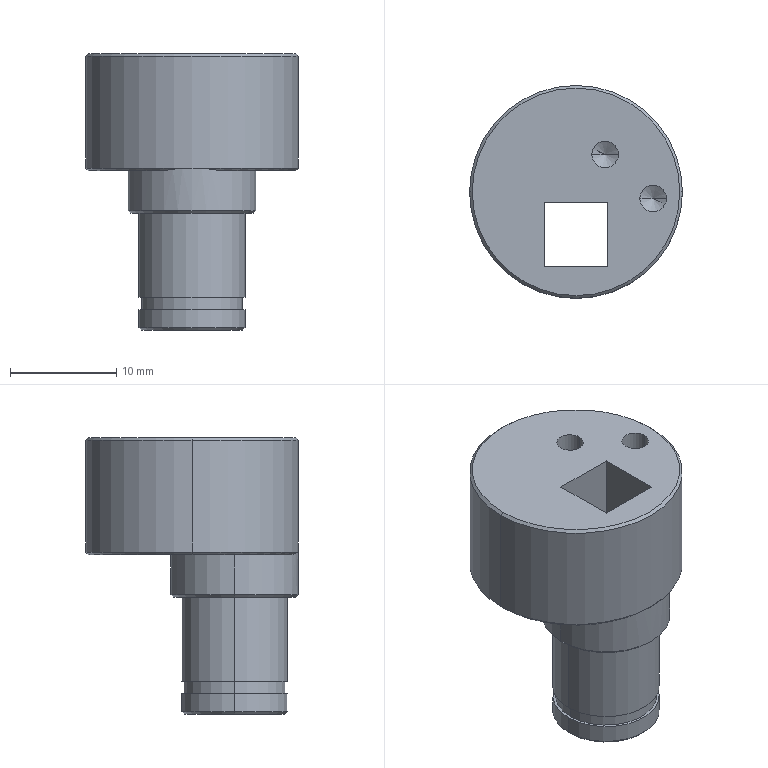Part | NX | features BREP 1 | 1 solid | 37 faces | box 20 x 20 x 26 mm | volume 3745 mm3 | cylinder 14 | cone 13 | plane 10 | commonest cylinder face diameters 2.5 x4 10 x4 9.5 x2 12 x2 20 x2
STEP:
#1=CARTESIAN_POINT('',(1.486,3.518,11.));
#2=VERTEX_POINT('',#1);
#3=CARTESIAN_POINT('',(1.486,3.518,3.5));
#4=VERTEX_POINT('',#3);
#5=CARTESIAN_POINT('',(1.486,3.518,11.));
#6=DIRECTION('',(0.,0.,1.));
#7=VECTOR('',#6,1000.);
#8=LINE('',#5,#7);
#9=EDGE_CURVE('',#2,#4,#8,.F.);
#10=ORIENTED_EDGE('',*,*,#9,.T.);
#11=CARTESIAN_POINT('',(3.986,3.518,3.5));
#12=VERTEX_POINT('',#11);
#13=CARTESIAN_POINT('',(2.736,3.518,3.5));
#14=DIRECTION('',(0.,0.,1.));
#15=DIRECTION('',(1.,0.,0.));
#16=AXIS2_PLACEMENT_3D('',#13,#14,#15);
#17=CIRCLE('',#16,1.25);
#18=EDGE_CURVE('',#12,#4,#17,.T.);
#19=ORIENTED_EDGE('',*,*,#18,.F.);
#20=CARTESIAN_POINT('',(3.986,3.518,11.));
#21=VERTEX_POINT('',#20);
#22=CARTESIAN_POINT('',(3.986,3.518,11.));
#23=DIRECTION('',(0.,0.,1.));
#24=VECTOR('',#23,1000.);
#25=LINE('',#22,#24);
#26=EDGE_CURVE('',#21,#12,#25,.F.);
#27=ORIENTED_EDGE('',*,*,#26,.F.);
#28=CARTESIAN_POINT('',(2.736,3.518,11.));
#29=DIRECTION('',(0.,0.,1.));
#30=DIRECTION('',(1.,0.,0.));
#31=AXIS2_PLACEMENT_3D('',#28,#29,#30);
#32=CIRCLE('',#31,1.25);
#33=EDGE_CURVE('',#21,#2,#32,.T.);
#34=ORIENTED_EDGE('',*,*,#33,.T.);
#35=EDGE_LOOP('',(#10,#19,#27,#34));
#36=FACE_BOUND('',#35,.T.);
#37=CARTESIAN_POINT('',(2.736,3.518,11.));
#38=DIRECTION('',(0.,0.,1.));
#39=DIRECTION('',(1.,0.,0.));
#40=AXIS2_PLACEMENT_3D('',#37,#38,#39);
#41=CYLINDRICAL_SURFACE('',#40,1.25);
#42=ADVANCED_FACE('',(#36),#41,.F.);
#43=CARTESIAN_POINT('',(2.736,3.518,2.749));
#44=VERTEX_POINT('',#43);
#45=CARTESIAN_POINT('',(1.486,3.518,3.5));
#46=DIRECTION('',(-0.8572,0.,0.515));
#47=VECTOR('',#46,1000.);
#48=LINE('',#45,#47);
#49=EDGE_CURVE('',#44,#4,#48,.T.);
#50=ORIENTED_EDGE('',*,*,#49,.F.);
#51=CARTESIAN_POINT('',(3.986,3.518,3.5));
#52=DIRECTION('',(0.8572,0.,0.515));
#53=VECTOR('',#52,1000.);
#54=LINE('',#51,#53);
#55=EDGE_CURVE('',#44,#12,#54,.T.);
#56=ORIENTED_EDGE('',*,*,#55,.T.);
#57=ORIENTED_EDGE('',*,*,#18,.T.);
#58=EDGE_LOOP('',(#50,#56,#57));
#59=FACE_BOUND('',#58,.T.);
#60=CARTESIAN_POINT('',(2.736,3.518,3.5));
#61=DIRECTION('',(0.,0.,1.));
#62=DIRECTION('',(1.,0.,0.));
#63=AXIS2_PLACEMENT_3D('',#60,#61,#62);
#64=CONICAL_SURFACE('',#63,1.25,1.03);
#65=ADVANCED_FACE('',(#59),#64,.F.);
#66=CARTESIAN_POINT('',(6.,-0.6191,11.));
#67=VERTEX_POINT('',#66);
#68=CARTESIAN_POINT('',(6.,-0.6191,3.5));
#69=VERTEX_POINT('',#68);
#70=CARTESIAN_POINT('',(6.,-0.6191,11.));
#71=DIRECTION('',(0.,0.,1.));
#72=VECTOR('',#71,1000.);
#73=LINE('',#70,#72);
#74=EDGE_CURVE('',#67,#69,#73,.F.);
#75=ORIENTED_EDGE('',*,*,#74,.T.);
#76=CARTESIAN_POINT('',(8.5,-0.6191,3.5));
#77=VERTEX_POINT('',#76);
#78=CARTESIAN_POINT('',(7.25,-0.6191,3.5));
#79=DIRECTION('',(0.,0.,1.));
#80=DIRECTION('',(1.,0.,0.));
#81=AXIS2_PLACEMENT_3D('',#78,#79,#80);
#82=CIRCLE('',#81,1.25);
#83=EDGE_CURVE('',#77,#69,#82,.T.);
#84=ORIENTED_EDGE('',*,*,#83,.F.);
#85=CARTESIAN_POINT('',(8.5,-0.6191,11.));
#86=VERTEX_POINT('',#85);
#87=CARTESIAN_POINT('',(8.5,-0.6191,11.));
#88=DIRECTION('',(0.,0.,1.));
#89=VECTOR('',#88,1000.);
#90=LINE('',#87,#89);
#91=EDGE_CURVE('',#86,#77,#90,.F.);
#92=ORIENTED_EDGE('',*,*,#91,.F.);
#93=CARTESIAN_POINT('',(7.25,-0.6191,11.));
#94=DIRECTION('',(0.,0.,1.));
#95=DIRECTION('',(1.,0.,0.));
#96=AXIS2_PLACEMENT_3D('',#93,#94,#95);
#97=CIRCLE('',#96,1.25);
#98=EDGE_CURVE('',#86,#67,#97,.T.);
#99=ORIENTED_EDGE('',*,*,#98,.T.);
#100=EDGE_LOOP('',(#75,#84,#92,#99));
#101=FACE_BOUND('',#100,.T.);
#102=CARTESIAN_POINT('',(7.25,-0.6191,11.));
#103=DIRECTION('',(0.,0.,1.));
#104=DIRECTION('',(1.,0.,0.));
#105=AXIS2_PLACEMENT_3D('',#102,#103,#104);
#106=CYLINDRICAL_SURFACE('',#105,1.25);
#107=ADVANCED_FACE('',(#101),#106,.F.);
#108=CARTESIAN_POINT('',(7.25,-0.6191,2.749));
#109=VERTEX_POINT('',#108);
#110=CARTESIAN_POINT('',(6.,-0.6191,3.5));
#111=DIRECTION('',(-0.8572,0.,0.515));
#112=VECTOR('',#111,1000.);
#113=LINE('',#110,#112);
#114=EDGE_CURVE('',#109,#69,#113,.T.);
#115=ORIENTED_EDGE('',*,*,#114,.F.);
#116=CARTESIAN_POINT('',(8.5,-0.6191,3.5));
#117=DIRECTION('',(0.8572,0.,0.515));
#118=VECTOR('',#117,1000.);
#119=LINE('',#116,#118);
#120=EDGE_CURVE('',#109,#77,#119,.T.);
#121=ORIENTED_EDGE('',*,*,#120,.T.);
#122=ORIENTED_EDGE('',*,*,#83,.T.);
#123=EDGE_LOOP('',(#115,#121,#122));
#124=FACE_BOUND('',#123,.T.);
#125=CARTESIAN_POINT('',(7.25,-0.6191,3.5));
#126=DIRECTION('',(0.,0.,1.));
#127=DIRECTION('',(1.,0.,0.));
#128=AXIS2_PLACEMENT_3D('',#125,#126,#127);
#129=CONICAL_SURFACE('',#128,1.25,1.03);
#130=ADVANCED_FACE('',(#124),#129,.F.);
#131=CARTESIAN_POINT('',(9.75,0.,11.));
#132=VERTEX_POINT('',#131);
#133=CARTESIAN_POINT('',(10.,0.,10.75));
#134=VERTEX_POINT('',#133);
#135=CARTESIAN_POINT('',(9.75,0.,11.));
#136=DIRECTION('',(0.7071,0.,-0.7071));
#137=VECTOR('',#136,1000.);
#138=LINE('',#135,#137);
#139=EDGE_CURVE('',#132,#134,#138,.T.);
#140=ORIENTED_EDGE('',*,*,#139,.F.);
#141=CARTESIAN_POINT('',(-9.75,0.,11.));
#142=VERTEX_POINT('',#141);
#143=CARTESIAN_POINT('',(0.,0.,11.));
#144=DIRECTION('',(0.,0.,1.));
#145=DIRECTION('',(1.,0.,0.));
#146=AXIS2_PLACEMENT_3D('',#143,#144,#145);
#147=CIRCLE('',#146,9.75);
#148=EDGE_CURVE('',#142,#132,#147,.T.);
#149=ORIENTED_EDGE('',*,*,#148,.F.);
#150=CARTESIAN_POINT('',(-10.,0.,10.75));
#151=VERTEX_POINT('',#150);
#152=CARTESIAN_POINT('',(-9.75,0.,11.));
#153=DIRECTION('',(-0.7071,0.,-0.7071));
#154=VECTOR('',#153,1000.);
#155=LINE('',#152,#154);
#156=EDGE_CURVE('',#142,#151,#155,.T.);
#157=ORIENTED_EDGE('',*,*,#156,.T.);
#158=CARTESIAN_POINT('',(0.,0.,10.75));
#159=DIRECTION('',(0.,0.,-1.));
#160=DIRECTION('',(1.,0.,0.));
#161=AXIS2_PLACEMENT_3D('',#158,#159,#160);
#162=CIRCLE('',#161,10.);
#163=EDGE_CURVE('',#134,#151,#162,.T.);
#164=ORIENTED_EDGE('',*,*,#163,.F.);
#165=EDGE_LOOP('',(#140,#149,#157,#164));
#166=FACE_BOUND('',#165,.T.);
#167=CARTESIAN_POINT('',(0.,0.,11.));
#168=DIRECTION('',(0.,0.,-1.));
#169=DIRECTION('',(-1.,0.,0.));
#170=AXIS2_PLACEMENT_3D('',#167,#168,#169);
#171=CONICAL_SURFACE('',#170,9.75,0.7854);
#172=ADVANCED_FACE('',(#166),#171,.T.);
#173=CARTESIAN_POINT('',(-9.75,0.,0.));
#174=VERTEX_POINT('',#173);
#175=CARTESIAN_POINT('',(-10.,0.,0.25));
#176=VERTEX_POINT('',#175);
#177=CARTESIAN_POINT('',(-10.,0.,0.25));
#178=DIRECTION('',(-0.7071,0.,0.7071));
#179=VECTOR('',#178,1000.);
#180=LINE('',#177,#179);
#181=EDGE_CURVE('',#174,#176,#180,.T.);
#182=ORIENTED_EDGE('',*,*,#181,.F.);
#183=CARTESIAN_POINT('',(-2.651,-9.383,0.));
#184=VERTEX_POINT('',#183);
#185=CARTESIAN_POINT('',(0.,0.,0.));
#186=DIRECTION('',(0.,0.,-1.));
#187=DIRECTION('',(1.,0.,0.));
#188=AXIS2_PLACEMENT_3D('',#185,#186,#187);
#189=CIRCLE('',#188,9.75);
#190=EDGE_CURVE('',#184,#174,#189,.T.);
#191=ORIENTED_EDGE('',*,*,#190,.F.);
#192=CARTESIAN_POINT('',(0.,-10.,0.25));
#193=VERTEX_POINT('',#192);
#194=CARTESIAN_POINT('',(0.,-10.,0.25));
#195=CARTESIAN_POINT('',(-0.9106,-10.,0.25));
#196=CARTESIAN_POINT('',(-1.826,-9.789,0.1667));
#197=CARTESIAN_POINT('',(-2.651,-9.383,0.));
#198=B_SPLINE_CURVE_WITH_KNOTS('',3,(#194,#195,#196,#197),.UNSPECIFIED.,.F.,.F.,(4,4),(0.,1.),.UNSPECIFIED.);
#199=EDGE_CURVE('',#193,#184,#198,.T.);
#200=ORIENTED_EDGE('',*,*,#199,.F.);
#201=CARTESIAN_POINT('',(0.,0.,0.25));
#202=DIRECTION('',(0.,0.,1.));
#203=DIRECTION('',(1.,0.,0.));
#204=AXIS2_PLACEMENT_3D('',#201,#202,#203);
#205=CIRCLE('',#204,10.);
#206=EDGE_CURVE('',#176,#193,#205,.T.);
#207=ORIENTED_EDGE('',*,*,#206,.F.);
#208=EDGE_LOOP('',(#182,#191,#200,#207));
#209=FACE_BOUND('',#208,.T.);
#210=CARTESIAN_POINT('',(0.,0.,0.25));
#211=DIRECTION('',(0.,0.,1.));
#212=DIRECTION('',(1.,0.,0.));
#213=AXIS2_PLACEMENT_3D('',#210,#211,#212);
#214=CONICAL_SURFACE('',#213,10.,0.7854);
#215=ADVANCED_FACE('',(#209),#214,.T.);
#216=CARTESIAN_POINT('',(-6.,-4.,-3.75));
#217=VERTEX_POINT('',#216);
#218=CARTESIAN_POINT('',(-5.75,-4.,-4.));
#219=VERTEX_POINT('',#218);
#220=CARTESIAN_POINT('',(-5.75,-4.,-4.));
#221=DIRECTION('',(-0.7071,0.,0.7071));
#222=VECTOR('',#221,1000.);
#223=LINE('',#220,#222);
#224=EDGE_CURVE('',#217,#219,#223,.F.);
#225=ORIENTED_EDGE('',*,*,#224,.T.);
#226=CARTESIAN_POINT('',(5.75,-4.,-4.));
#227=VERTEX_POINT('',#226);
#228=CARTESIAN_POINT('',(0.,-4.,-4.));
#229=DIRECTION('',(0.,0.,-1.));
#230=DIRECTION('',(-1.,0.,0.));
#231=AXIS2_PLACEMENT_3D('',#228,#229,#230);
#232=CIRCLE('',#231,5.75);
#233=EDGE_CURVE('',#227,#219,#232,.T.);
#234=ORIENTED_EDGE('',*,*,#233,.F.);
#235=CARTESIAN_POINT('',(6.,-4.,-3.75));
#236=VERTEX_POINT('',#235);
#237=CARTESIAN_POINT('',(5.75,-4.,-4.));
#238=DIRECTION('',(0.7071,0.,0.7071));
#239=VECTOR('',#238,1000.);
#240=LINE('',#237,#239);
#241=EDGE_CURVE('',#236,#227,#240,.F.);
#242=ORIENTED_EDGE('',*,*,#241,.F.);
#243=CARTESIAN_POINT('',(0.,-4.,-3.75));
#244=DIRECTION('',(0.,0.,1.));
#245=DIRECTION('',(-1.,0.,0.));
#246=AXIS2_PLACEMENT_3D('',#243,#244,#245);
#247=CIRCLE('',#246,6.);
#248=EDGE_CURVE('',#217,#236,#247,.T.);
#249=ORIENTED_EDGE('',*,*,#248,.F.);
#250=EDGE_LOOP('',(#225,#234,#242,#249));
#251=FACE_BOUND('',#250,.T.);
#252=CARTESIAN_POINT('',(0.,-4.,-4.));
#253=DIRECTION('',(0.,0.,1.));
#254=DIRECTION('',(1.,0.,0.));
#255=AXIS2_PLACEMENT_3D('',#252,#253,#254);
#256=CONICAL_SURFACE('',#255,5.75,0.7854);
#257=ADVANCED_FACE('',(#251),#256,.T.);
#258=CARTESIAN_POINT('',(-5.,-4.,-14.75));
#259=VERTEX_POINT('',#258);
#260=CARTESIAN_POINT('',(-4.75,-4.,-15.));
#261=VERTEX_POINT('',#260);
#262=CARTESIAN_POINT('',(-4.75,-4.,-15.));
#263=DIRECTION('',(-0.7071,0.,0.7071));
#264=VECTOR('',#263,1000.);
#265=LINE('',#262,#264);
#266=EDGE_CURVE('',#259,#261,#265,.F.);
#267=ORIENTED_EDGE('',*,*,#266,.T.);
#268=CARTESIAN_POINT('',(4.75,-4.,-15.));
#269=VERTEX_POINT('',#268);
#270=CARTESIAN_POINT('',(0.,-4.,-15.));
#271=DIRECTION('',(0.,0.,-1.));
#272=DIRECTION('',(-1.,0.,0.));
#273=AXIS2_PLACEMENT_3D('',#270,#271,#272);
#274=CIRCLE('',#273,4.75);
#275=EDGE_CURVE('',#269,#261,#274,.T.);
#276=ORIENTED_EDGE('',*,*,#275,.F.);
#277=CARTESIAN_POINT('',(5.,-4.,-14.75));
#278=VERTEX_POINT('',#277);
#279=CARTESIAN_POINT('',(4.75,-4.,-15.));
#280=DIRECTION('',(0.7071,0.,0.7071));
#281=VECTOR('',#280,1000.);
#282=LINE('',#279,#281);
#283=EDGE_CURVE('',#278,#269,#282,.F.);
#284=ORIENTED_EDGE('',*,*,#283,.F.);
#285=CARTESIAN_POINT('',(0.,-4.,-14.75));
#286=DIRECTION('',(0.,0.,1.));
#287=DIRECTION('',(-1.,0.,0.));
#288=AXIS2_PLACEMENT_3D('',#285,#286,#287);
#289=CIRCLE('',#288,5.);
#290=EDGE_CURVE('',#259,#278,#289,.T.);
#291=ORIENTED_EDGE('',*,*,#290,.F.);
#292=EDGE_LOOP('',(#267,#276,#284,#291));
#293=FACE_BOUND('',#292,.T.);
#294=CARTESIAN_POINT('',(0.,-4.,-15.));
#295=DIRECTION('',(0.,0.,1.));
#296=DIRECTION('',(1.,0.,0.));
#297=AXIS2_PLACEMENT_3D('',#294,#295,#296);
#298=CONICAL_SURFACE('',#297,4.75,0.7854);
#299=ADVANCED_FACE('',(#293),#298,.T.);
#300=CARTESIAN_POINT('',(-4.75,-4.,-11.9));
#301=VERTEX_POINT('',#300);
#302=CARTESIAN_POINT('',(-4.75,-4.,-13.05));
#303=VERTEX_POINT('',#302);
#304=CARTESIAN_POINT('',(-4.75,-4.,-13.05));
#305=DIRECTION('',(0.,0.,1.));
#306=VECTOR('',#305,1000.);
#307=LINE('',#304,#306);
#308=EDGE_CURVE('',#301,#303,#307,.F.);
#309=ORIENTED_EDGE('',*,*,#308,.T.);
#310=CARTESIAN_POINT('',(4.75,-4.,-13.05));
#311=VERTEX_POINT('',#310);
#312=CARTESIAN_POINT('',(0.,-4.,-13.05));
#313=DIRECTION('',(0.,0.,-1.));
#314=DIRECTION('',(-1.,0.,0.));
#315=AXIS2_PLACEMENT_3D('',#312,#313,#314);
#316=CIRCLE('',#315,4.75);
#317=EDGE_CURVE('',#311,#303,#316,.T.);
#318=ORIENTED_EDGE('',*,*,#317,.F.);
#319=CARTESIAN_POINT('',(4.75,-4.,-11.9));
#320=VERTEX_POINT('',#319);
#321=CARTESIAN_POINT('',(4.75,-4.,-13.05));
#322=DIRECTION('',(0.,0.,1.));
#323=VECTOR('',#322,1000.);
#324=LINE('',#321,#323);
#325=EDGE_CURVE('',#320,#311,#324,.F.);
#326=ORIENTED_EDGE('',*,*,#325,.F.);
#327=CARTESIAN_POINT('',(0.,-4.,-11.9));
#328=DIRECTION('',(0.,0.,-1.));
#329=DIRECTION('',(-1.,0.,0.));
#330=AXIS2_PLACEMENT_3D('',#327,#328,#329);
#331=CIRCLE('',#330,4.75);
#332=EDGE_CURVE('',#320,#301,#331,.T.);
#333=ORIENTED_EDGE('',*,*,#332,.T.);
#334=EDGE_LOOP('',(#309,#318,#326,#333));
#335=FACE_BOUND('',#334,.T.);
#336=CARTESIAN_POINT('',(0.,-4.,-13.05));
#337=DIRECTION('',(0.,0.,1.));
#338=DIRECTION('',(1.,0.,0.));
#339=AXIS2_PLACEMENT_3D('',#336,#337,#338);
#340=CYLINDRICAL_SURFACE('',#339,4.75);
#341=ADVANCED_FACE('',(#335),#340,.T.);
#342=CARTESIAN_POINT('',(5.,-4.,-11.9));
#343=VERTEX_POINT('',#342);
#344=CARTESIAN_POINT('',(-5.,-4.,-11.9));
#345=VERTEX_POINT('',#344);
#346=CARTESIAN_POINT('',(0.,-4.,-11.9));
#347=DIRECTION('',(0.,0.,-1.));
#348=DIRECTION('',(-1.,0.,0.));
#349=AXIS2_PLACEMENT_3D('',#346,#347,#348);
#350=CIRCLE('',#349,5.);
#351=EDGE_CURVE('',#343,#345,#350,.T.);
#352=ORIENTED_EDGE('',*,*,#351,.T.);
#353=CARTESIAN_POINT('',(0.,-4.,-11.9));
#354=DIRECTION('',(0.,0.,-1.));
#355=DIRECTION('',(-1.,0.,0.));
#356=AXIS2_PLACEMENT_3D('',#353,#354,#355);
#357=CIRCLE('',#356,5.);
#358=EDGE_CURVE('',#345,#343,#357,.T.);
#359=ORIENTED_EDGE('',*,*,#358,.T.);
#360=EDGE_LOOP('',(#352,#359));
#361=FACE_BOUND('',#360,.T.);
#362=ORIENTED_EDGE('',*,*,#332,.F.);
#363=CARTESIAN_POINT('',(0.,-4.,-11.9));
#364=DIRECTION('',(0.,0.,-1.));
#365=DIRECTION('',(-1.,0.,0.));
#366=AXIS2_PLACEMENT_3D('',#363,#364,#365);
#367=CIRCLE('',#366,4.75);
#368=EDGE_CURVE('',#301,#320,#367,.T.);
#369=ORIENTED_EDGE('',*,*,#368,.F.);
#370=EDGE_LOOP('',(#362,#369));
#371=FACE_BOUND('',#370,.T.);
#372=CARTESIAN_POINT('',(0.,-4.,-11.9));
#373=DIRECTION('',(0.,0.,-1.));
#374=DIRECTION('',(-1.,0.,0.));
#375=AXIS2_PLACEMENT_3D('',#372,#373,#374);
#376=PLANE('',#375);
#377=ADVANCED_FACE('',(#361,#371),#376,.T.);
#378=CARTESIAN_POINT('',(5.,-4.,-13.05));
#379=VERTEX_POINT('',#378);
#380=CARTESIAN_POINT('',(-5.,-4.,-13.05));
#381=VERTEX_POINT('',#380);
#382=CARTESIAN_POINT('',(0.,-4.,-13.05));
#383=DIRECTION('',(0.,0.,-1.));
#384=DIRECTION('',(-1.,0.,0.));
#385=AXIS2_PLACEMENT_3D('',#382,#383,#384);
#386=CIRCLE('',#385,5.);
#387=EDGE_CURVE('',#379,#381,#386,.T.);
#388=ORIENTED_EDGE('',*,*,#387,.F.);
#389=CARTESIAN_POINT('',(0.,-4.,-13.05));
#390=DIRECTION('',(0.,0.,-1.));
#391=DIRECTION('',(-1.,0.,0.));
#392=AXIS2_PLACEMENT_3D('',#389,#390,#391);
#393=CIRCLE('',#392,5.);
#394=EDGE_CURVE('',#381,#379,#393,.T.);
#395=ORIENTED_EDGE('',*,*,#394,.F.);
#396=EDGE_LOOP('',(#388,#395));
#397=FACE_BOUND('',#396,.T.);
#398=ORIENTED_EDGE('',*,*,#317,.T.);
#399=CARTESIAN_POINT('',(0.,-4.,-13.05));
#400=DIRECTION('',(0.,0.,-1.));
#401=DIRECTION('',(-1.,0.,0.));
#402=AXIS2_PLACEMENT_3D('',#399,#400,#401);
#403=CIRCLE('',#402,4.75);
#404=EDGE_CURVE('',#303,#311,#403,.T.);
#405=ORIENTED_EDGE('',*,*,#404,.T.);
#406=EDGE_LOOP('',(#398,#405));
#407=FACE_BOUND('',#406,.T.);
#408=CARTESIAN_POINT('',(0.,-4.,-13.05));
#409=DIRECTION('',(0.,0.,-1.));
#410=DIRECTION('',(-1.,0.,0.));
#411=AXIS2_PLACEMENT_3D('',#408,#409,#410);
#412=PLANE('',#411);
#413=ADVANCED_FACE('',(#397,#407),#412,.F.);
#414=CARTESIAN_POINT('',(-3.,-1.,-15.));
#415=VERTEX_POINT('',#414);
#416=CARTESIAN_POINT('',(3.,-1.,-15.));
#417=VERTEX_POINT('',#416);
#418=CARTESIAN_POINT('',(3.,-1.,-15.));
#419=DIRECTION('',(1.,0.,0.));
#420=VECTOR('',#419,1000.);
#421=LINE('',#418,#420);
#422=EDGE_CURVE('',#415,#417,#421,.T.);
#423=ORIENTED_EDGE('',*,*,#422,.T.);
#424=CARTESIAN_POINT('',(3.,-1.,11.));
#425=VERTEX_POINT('',#424);
#426=CARTESIAN_POINT('',(3.,-1.,11.));
#427=DIRECTION('',(0.,0.,-1.));
#428=VECTOR('',#427,1000.);
#429=LINE('',#426,#428);
#430=EDGE_CURVE('',#425,#417,#429,.T.);
#431=ORIENTED_EDGE('',*,*,#430,.F.);
#432=CARTESIAN_POINT('',(-3.,-1.,11.));
#433=VERTEX_POINT('',#432);
#434=CARTESIAN_POINT('',(3.,-1.,11.));
#435=DIRECTION('',(1.,0.,0.));
#436=VECTOR('',#435,1000.);
#437=LINE('',#434,#436);
#438=EDGE_CURVE('',#433,#425,#437,.T.);
#439=ORIENTED_EDGE('',*,*,#438,.F.);
#440=CARTESIAN_POINT('',(-3.,-1.,11.));
#441=DIRECTION('',(0.,0.,-1.));
#442=VECTOR('',#441,1000.);
#443=LINE('',#440,#442);
#444=EDGE_CURVE('',#433,#415,#443,.T.);
#445=ORIENTED_EDGE('',*,*,#444,.T.);
#446=EDGE_LOOP('',(#423,#431,#439,#445));
#447=FACE_BOUND('',#446,.T.);
#448=CARTESIAN_POINT('',(3.,-1.,11.));
#449=DIRECTION('',(0.,1.,0.));
#450=DIRECTION('',(0.,0.,1.));
#451=AXIS2_PLACEMENT_3D('',#448,#449,#450);
#452=PLANE('',#451);
#453=ADVANCED_FACE('',(#447),#452,.F.);
#454=CARTESIAN_POINT('',(3.,-7.,-15.));
#455=VERTEX_POINT('',#454);
#456=CARTESIAN_POINT('',(3.,-7.,-15.));
#457=DIRECTION('',(0.,-1.,0.));
#458=VECTOR('',#457,1000.);
#459=LINE('',#456,#458);
#460=EDGE_CURVE('',#417,#455,#459,.T.);
#461=ORIENTED_EDGE('',*,*,#460,.T.);
#462=CARTESIAN_POINT('',(3.,-7.,11.));
#463=VERTEX_POINT('',#462);
#464=CARTESIAN_POINT('',(3.,-7.,11.));
#465=DIRECTION('',(0.,0.,-1.));
#466=VECTOR('',#465,1000.);
#467=LINE('',#464,#466);
#468=EDGE_CURVE('',#463,#455,#467,.T.);
#469=ORIENTED_EDGE('',*,*,#468,.F.);
#470=CARTESIAN_POINT('',(3.,-7.,11.));
#471=DIRECTION('',(0.,-1.,0.));
#472=VECTOR('',#471,1000.);
#473=LINE('',#470,#472);
#474=EDGE_CURVE('',#425,#463,#473,.T.);
#475=ORIENTED_EDGE('',*,*,#474,.F.);
#476=ORIENTED_EDGE('',*,*,#430,.T.);
#477=EDGE_LOOP('',(#461,#469,#475,#476));
#478=FACE_BOUND('',#477,.T.);
#479=CARTESIAN_POINT('',(3.,-7.,11.));
#480=DIRECTION('',(1.,0.,0.));
#481=DIRECTION('',(0.,0.,-1.));
#482=AXIS2_PLACEMENT_3D('',#479,#480,#481);
#483=PLANE('',#482);
#484=ADVANCED_FACE('',(#478),#483,.F.);
#485=CARTESIAN_POINT('',(-3.,-7.,-15.));
#486=VERTEX_POINT('',#485);
#487=CARTESIAN_POINT('',(3.,-7.,-15.));
#488=DIRECTION('',(-1.,0.,0.));
#489=VECTOR('',#488,1000.);
#490=LINE('',#487,#489);
#491=EDGE_CURVE('',#455,#486,#490,.T.);
#492=ORIENTED_EDGE('',*,*,#491,.T.);
#493=CARTESIAN_POINT('',(-3.,-7.,11.));
#494=VERTEX_POINT('',#493);
#495=CARTESIAN_POINT('',(-3.,-7.,11.));
#496=DIRECTION('',(0.,0.,-1.));
#497=VECTOR('',#496,1000.);
#498=LINE('',#495,#497);
#499=EDGE_CURVE('',#494,#486,#498,.T.);
#500=ORIENTED_EDGE('',*,*,#499,.F.);
#501=CARTESIAN_POINT('',(3.,-7.,11.));
#502=DIRECTION('',(-1.,0.,0.));
#503=VECTOR('',#502,1000.);
#504=LINE('',#501,#503);
#505=EDGE_CURVE('',#463,#494,#504,.T.);
#506=ORIENTED_EDGE('',*,*,#505,.F.);
#507=ORIENTED_EDGE('',*,*,#468,.T.);
#508=EDGE_LOOP('',(#492,#500,#506,#507));
#509=FACE_BOUND('',#508,.T.);
#510=CARTESIAN_POINT('',(3.,-7.,11.));
#511=DIRECTION('',(0.,-1.,0.));
#512=DIRECTION('',(0.,0.,-1.));
#513=AXIS2_PLACEMENT_3D('',#510,#511,#512);
#514=PLANE('',#513);
#515=ADVANCED_FACE('',(#509),#514,.F.);
#516=CARTESIAN_POINT('',(-3.,-7.,-15.));
#517=DIRECTION('',(0.,1.,0.));
#518=VECTOR('',#517,1000.);
#519=LINE('',#516,#518);
#520=EDGE_CURVE('',#486,#415,#519,.T.);
#521=ORIENTED_EDGE('',*,*,#520,.T.);
#522=ORIENTED_EDGE('',*,*,#444,.F.);
#523=CARTESIAN_POINT('',(-3.,-7.,11.));
#524=DIRECTION('',(0.,1.,0.));
#525=VECTOR('',#524,1000.);
#526=LINE('',#523,#525);
#527=EDGE_CURVE('',#494,#433,#526,.T.);
#528=ORIENTED_EDGE('',*,*,#527,.F.);
#529=ORIENTED_EDGE('',*,*,#499,.T.);
#530=EDGE_LOOP('',(#521,#522,#528,#529));
#531=FACE_BOUND('',#530,.T.);
#532=CARTESIAN_POINT('',(-3.,-7.,11.));
#533=DIRECTION('',(-1.,0.,0.));
#534=DIRECTION('',(0.,0.,1.));
#535=AXIS2_PLACEMENT_3D('',#532,#533,#534);
#536=PLANE('',#535);
#537=ADVANCED_FACE('',(#531),#536,.F.);
#538=CARTESIAN_POINT('',(-5.,-4.,-15.));
#539=DIRECTION('',(0.,0.,1.));
#540=VECTOR('',#539,1000.);
#541=LINE('',#538,#540);
#542=EDGE_CURVE('',#381,#259,#541,.F.);
#543=ORIENTED_EDGE('',*,*,#542,.T.);
#544=ORIENTED_EDGE('',*,*,#290,.T.);
#545=CARTESIAN_POINT('',(5.,-4.,-15.));
#546=DIRECTION('',(0.,0.,1.));
#547=VECTOR('',#546,1000.);
#548=LINE('',#545,#547);
#549=EDGE_CURVE('',#379,#278,#548,.F.);
#550=ORIENTED_EDGE('',*,*,#549,.F.);
#551=ORIENTED_EDGE('',*,*,#387,.T.);
#552=EDGE_LOOP('',(#543,#544,#550,#551));
#553=FACE_BOUND('',#552,.T.);
#554=CARTESIAN_POINT('',(0.,-4.,-15.));
#555=DIRECTION('',(0.,0.,1.));
#556=DIRECTION('',(1.,0.,0.));
#557=AXIS2_PLACEMENT_3D('',#554,#555,#556);
#558=CYLINDRICAL_SURFACE('',#557,5.);
#559=ADVANCED_FACE('',(#553),#558,.T.);
#560=ORIENTED_EDGE('',*,*,#520,.F.);
#561=ORIENTED_EDGE('',*,*,#491,.F.);
#562=ORIENTED_EDGE('',*,*,#460,.F.);
#563=ORIENTED_EDGE('',*,*,#422,.F.);
#564=EDGE_LOOP('',(#560,#561,#562,#563));
#565=FACE_BOUND('',#564,.T.);
#566=ORIENTED_EDGE('',*,*,#275,.T.);
#567=CARTESIAN_POINT('',(0.,-4.,-15.));
#568=DIRECTION('',(0.,0.,-1.));
#569=DIRECTION('',(-1.,0.,0.));
#570=AXIS2_PLACEMENT_3D('',#567,#568,#569);
#571=CIRCLE('',#570,4.75);
#572=EDGE_CURVE('',#261,#269,#571,.T.);
#573=ORIENTED_EDGE('',*,*,#572,.T.);
#574=EDGE_LOOP('',(#566,#573));
#575=FACE_BOUND('',#574,.T.);
#576=CARTESIAN_POINT('',(0.,-4.,-15.));
#577=DIRECTION('',(0.,0.,-1.));
#578=DIRECTION('',(-1.,0.,0.));
#579=AXIS2_PLACEMENT_3D('',#576,#577,#578);
#580=PLANE('',#579);
#581=ADVANCED_FACE('',(#565,#575),#580,.T.);
#582=CARTESIAN_POINT('',(-6.,-4.,0.));
#583=VERTEX_POINT('',#582);
#584=CARTESIAN_POINT('',(-6.,-4.,-4.));
#585=DIRECTION('',(0.,0.,1.));
#586=VECTOR('',#585,1000.);
#587=LINE('',#584,#586);
#588=EDGE_CURVE('',#583,#217,#587,.F.);
#589=ORIENTED_EDGE('',*,*,#588,.T.);
#590=ORIENTED_EDGE('',*,*,#248,.T.);
#591=CARTESIAN_POINT('',(6.,-4.,0.));
#592=VERTEX_POINT('',#591);
#593=CARTESIAN_POINT('',(6.,-4.,-4.));
#594=DIRECTION('',(0.,0.,1.));
#595=VECTOR('',#594,1000.);
#596=LINE('',#593,#595);
#597=EDGE_CURVE('',#592,#236,#596,.F.);
#598=ORIENTED_EDGE('',*,*,#597,.F.);
#599=CARTESIAN_POINT('',(2.651,-9.383,0.));
#600=VERTEX_POINT('',#599);
#601=CARTESIAN_POINT('',(0.,-4.,0.));
#602=DIRECTION('',(0.,0.,-1.));
#603=DIRECTION('',(-1.,0.,0.));
#604=AXIS2_PLACEMENT_3D('',#601,#602,#603);
#605=CIRCLE('',#604,6.);
#606=EDGE_CURVE('',#592,#600,#605,.T.);
#607=ORIENTED_EDGE('',*,*,#606,.T.);
#608=CARTESIAN_POINT('',(2.651,-9.383,0.));
#609=CARTESIAN_POINT('',(1.826,-9.789,0.1667));
#610=CARTESIAN_POINT('',(0.9106,-10.,0.25));
#611=CARTESIAN_POINT('',(0.,-10.,0.25));
#612=B_SPLINE_CURVE_WITH_KNOTS('',3,(#608,#609,#610,#611),.UNSPECIFIED.,.F.,.F.,(4,4),(0.,1.),.UNSPECIFIED.);
#613=EDGE_CURVE('',#600,#193,#612,.T.);
#614=ORIENTED_EDGE('',*,*,#613,.T.);
#615=ORIENTED_EDGE('',*,*,#199,.T.);
#616=CARTESIAN_POINT('',(0.,-4.,0.));
#617=DIRECTION('',(0.,0.,-1.));
#618=DIRECTION('',(-1.,0.,0.));
#619=AXIS2_PLACEMENT_3D('',#616,#617,#618);
#620=CIRCLE('',#619,6.);
#621=EDGE_CURVE('',#184,#583,#620,.T.);
#622=ORIENTED_EDGE('',*,*,#621,.T.);
#623=EDGE_LOOP('',(#589,#590,#598,#607,#614,#615,#622));
#624=FACE_BOUND('',#623,.T.);
#625=CARTESIAN_POINT('',(0.,-4.,-4.));
#626=DIRECTION('',(0.,0.,1.));
#627=DIRECTION('',(1.,0.,0.));
#628=AXIS2_PLACEMENT_3D('',#625,#626,#627);
#629=CYLINDRICAL_SURFACE('',#628,6.);
#630=ADVANCED_FACE('',(#624),#629,.T.);
#631=CARTESIAN_POINT('',(5.,-4.,-4.));
#632=VERTEX_POINT('',#631);
#633=CARTESIAN_POINT('',(-5.,-4.,-4.));
#634=VERTEX_POINT('',#633);
#635=CARTESIAN_POINT('',(0.,-4.,-4.));
#636=DIRECTION('',(0.,0.,-1.));
#637=DIRECTION('',(-1.,0.,0.));
#638=AXIS2_PLACEMENT_3D('',#635,#636,#637);
#639=CIRCLE('',#638,5.);
#640=EDGE_CURVE('',#632,#634,#639,.T.);
#641=ORIENTED_EDGE('',*,*,#640,.F.);
#642=CARTESIAN_POINT('',(0.,-4.,-4.));
#643=DIRECTION('',(0.,0.,-1.));
#644=DIRECTION('',(-1.,0.,0.));
#645=AXIS2_PLACEMENT_3D('',#642,#643,#644);
#646=CIRCLE('',#645,5.);
#647=EDGE_CURVE('',#634,#632,#646,.T.);
#648=ORIENTED_EDGE('',*,*,#647,.F.);
#649=EDGE_LOOP('',(#641,#648));
#650=FACE_BOUND('',#649,.T.);
#651=ORIENTED_EDGE('',*,*,#233,.T.);
#652=CARTESIAN_POINT('',(0.,-4.,-4.));
#653=DIRECTION('',(0.,0.,-1.));
#654=DIRECTION('',(-1.,0.,0.));
#655=AXIS2_PLACEMENT_3D('',#652,#653,#654);
#656=CIRCLE('',#655,5.75);
#657=EDGE_CURVE('',#219,#227,#656,.T.);
#658=ORIENTED_EDGE('',*,*,#657,.T.);
#659=EDGE_LOOP('',(#651,#658));
#660=FACE_BOUND('',#659,.T.);
#661=CARTESIAN_POINT('',(0.,-4.,-4.));
#662=DIRECTION('',(0.,0.,-1.));
#663=DIRECTION('',(-1.,0.,0.));
#664=AXIS2_PLACEMENT_3D('',#661,#662,#663);
#665=PLANE('',#664);
#666=ADVANCED_FACE('',(#650,#660),#665,.T.);
#667=ORIENTED_EDGE('',*,*,#527,.T.);
#668=ORIENTED_EDGE('',*,*,#438,.T.);
#669=ORIENTED_EDGE('',*,*,#474,.T.);
#670=ORIENTED_EDGE('',*,*,#505,.T.);
#671=EDGE_LOOP('',(#667,#668,#669,#670));
#672=FACE_BOUND('',#671,.T.);
#673=ORIENTED_EDGE('',*,*,#148,.T.);
#674=CARTESIAN_POINT('',(0.,0.,11.));
#675=DIRECTION('',(0.,0.,1.));
#676=DIRECTION('',(1.,0.,0.));
#677=AXIS2_PLACEMENT_3D('',#674,#675,#676);
#678=CIRCLE('',#677,9.75);
#679=EDGE_CURVE('',#132,#142,#678,.T.);
#680=ORIENTED_EDGE('',*,*,#679,.T.);
#681=EDGE_LOOP('',(#673,#680));
#682=FACE_BOUND('',#681,.T.);
#683=ORIENTED_EDGE('',*,*,#98,.F.);
#684=CARTESIAN_POINT('',(7.25,-0.6191,11.));
#685=DIRECTION('',(0.,0.,1.));
#686=DIRECTION('',(1.,0.,0.));
#687=AXIS2_PLACEMENT_3D('',#684,#685,#686);
#688=CIRCLE('',#687,1.25);
#689=EDGE_CURVE('',#67,#86,#688,.T.);
#690=ORIENTED_EDGE('',*,*,#689,.F.);
#691=EDGE_LOOP('',(#683,#690));
#692=FACE_BOUND('',#691,.T.);
#693=ORIENTED_EDGE('',*,*,#33,.F.);
#694=CARTESIAN_POINT('',(2.736,3.518,11.));
#695=DIRECTION('',(0.,0.,1.));
#696=DIRECTION('',(1.,0.,0.));
#697=AXIS2_PLACEMENT_3D('',#694,#695,#696);
#698=CIRCLE('',#697,1.25);
#699=EDGE_CURVE('',#2,#21,#698,.T.);
#700=ORIENTED_EDGE('',*,*,#699,.F.);
#701=EDGE_LOOP('',(#693,#700));
#702=FACE_BOUND('',#701,.T.);
#703=CARTESIAN_POINT('',(0.,0.,11.));
#704=DIRECTION('',(0.,0.,1.));
#705=DIRECTION('',(1.,0.,0.));
#706=AXIS2_PLACEMENT_3D('',#703,#704,#705);
#707=PLANE('',#706);
#708=ADVANCED_FACE('',(#672,#682,#692,#702),#707,.T.);
#709=CARTESIAN_POINT('',(10.,0.,0.25));
#710=VERTEX_POINT('',#709);
#711=CARTESIAN_POINT('',(10.,0.,11.));
#712=DIRECTION('',(0.,0.,-1.));
#713=VECTOR('',#712,1000.);
#714=LINE('',#711,#713);
#715=EDGE_CURVE('',#134,#710,#714,.T.);
#716=ORIENTED_EDGE('',*,*,#715,.F.);
#717=ORIENTED_EDGE('',*,*,#163,.T.);
#718=CARTESIAN_POINT('',(-10.,0.,11.));
#719=DIRECTION('',(0.,0.,-1.));
#720=VECTOR('',#719,1000.);
#721=LINE('',#718,#720);
#722=EDGE_CURVE('',#151,#176,#721,.T.);
#723=ORIENTED_EDGE('',*,*,#722,.T.);
#724=ORIENTED_EDGE('',*,*,#206,.T.);
#725=CARTESIAN_POINT('',(0.,0.,0.25));
#726=DIRECTION('',(0.,0.,1.));
#727=DIRECTION('',(1.,0.,0.));
#728=AXIS2_PLACEMENT_3D('',#725,#726,#727);
#729=CIRCLE('',#728,10.);
#730=EDGE_CURVE('',#193,#710,#729,.T.);
#731=ORIENTED_EDGE('',*,*,#730,.T.);
#732=EDGE_LOOP('',(#716,#717,#723,#724,#731));
#733=FACE_BOUND('',#732,.T.);
#734=CARTESIAN_POINT('',(0.,0.,11.));
#735=DIRECTION('',(0.,0.,-1.));
#736=DIRECTION('',(-1.,0.,0.));
#737=AXIS2_PLACEMENT_3D('',#734,#735,#736);
#738=CYLINDRICAL_SURFACE('',#737,10.);
#739=ADVANCED_FACE('',(#733),#738,.T.);
#740=ORIENTED_EDGE('',*,*,#621,.F.);
#741=ORIENTED_EDGE('',*,*,#190,.T.);
#742=CARTESIAN_POINT('',(9.75,0.,0.));
#743=VERTEX_POINT('',#742);
#744=CARTESIAN_POINT('',(0.,0.,0.));
#745=DIRECTION('',(0.,0.,-1.));
#746=DIRECTION('',(1.,0.,0.));
#747=AXIS2_PLACEMENT_3D('',#744,#745,#746);
#748=CIRCLE('',#747,9.75);
#749=EDGE_CURVE('',#174,#743,#748,.T.);
#750=ORIENTED_EDGE('',*,*,#749,.T.);
#751=CARTESIAN_POINT('',(0.,0.,0.));
#752=DIRECTION('',(0.,0.,-1.));
#753=DIRECTION('',(1.,0.,0.));
#754=AXIS2_PLACEMENT_3D('',#751,#752,#753);
#755=CIRCLE('',#754,9.75);
#756=EDGE_CURVE('',#743,#600,#755,.T.);
#757=ORIENTED_EDGE('',*,*,#756,.T.);
#758=ORIENTED_EDGE('',*,*,#606,.F.);
#759=CARTESIAN_POINT('',(0.,-4.,0.));
#760=DIRECTION('',(0.,0.,-1.));
#761=DIRECTION('',(-1.,0.,0.));
#762=AXIS2_PLACEMENT_3D('',#759,#760,#761);
#763=CIRCLE('',#762,6.);
#764=EDGE_CURVE('',#583,#592,#763,.T.);
#765=ORIENTED_EDGE('',*,*,#764,.F.);
#766=EDGE_LOOP('',(#740,#741,#750,#757,#758,#765));
#767=FACE_BOUND('',#766,.T.);
#768=CARTESIAN_POINT('',(0.,0.,0.));
#769=DIRECTION('',(0.,0.,1.));
#770=DIRECTION('',(1.,0.,0.));
#771=AXIS2_PLACEMENT_3D('',#768,#769,#770);
#772=PLANE('',#771);
#773=ADVANCED_FACE('',(#767),#772,.F.);
#774=CARTESIAN_POINT('',(-5.,-4.,-15.));
#775=DIRECTION('',(0.,0.,1.));
#776=VECTOR('',#775,1000.);
#777=LINE('',#774,#776);
#778=EDGE_CURVE('',#634,#345,#777,.F.);
#779=ORIENTED_EDGE('',*,*,#778,.T.);
#780=ORIENTED_EDGE('',*,*,#351,.F.);
#781=CARTESIAN_POINT('',(5.,-4.,-15.));
#782=DIRECTION('',(0.,0.,1.));
#783=VECTOR('',#782,1000.);
#784=LINE('',#781,#783);
#785=EDGE_CURVE('',#632,#343,#784,.F.);
#786=ORIENTED_EDGE('',*,*,#785,.F.);
#787=ORIENTED_EDGE('',*,*,#640,.T.);
#788=EDGE_LOOP('',(#779,#780,#786,#787));
#789=FACE_BOUND('',#788,.T.);
#790=CARTESIAN_POINT('',(0.,-4.,-15.));
#791=DIRECTION('',(0.,0.,1.));
#792=DIRECTION('',(1.,0.,0.));
#793=AXIS2_PLACEMENT_3D('',#790,#791,#792);
#794=CYLINDRICAL_SURFACE('',#793,5.);
#795=ADVANCED_FACE('',(#789),#794,.T.);
#796=ORIENTED_EDGE('',*,*,#358,.F.);
#797=ORIENTED_EDGE('',*,*,#778,.F.);
#798=ORIENTED_EDGE('',*,*,#647,.T.);
#799=ORIENTED_EDGE('',*,*,#785,.T.);
#800=EDGE_LOOP('',(#796,#797,#798,#799));
#801=FACE_BOUND('',#800,.T.);
#802=CARTESIAN_POINT('',(0.,-4.,-15.));
#803=DIRECTION('',(0.,0.,1.));
#804=DIRECTION('',(1.,0.,0.));
#805=AXIS2_PLACEMENT_3D('',#802,#803,#804);
#806=CYLINDRICAL_SURFACE('',#805,5.);
#807=ADVANCED_FACE('',(#801),#806,.T.);
#808=CARTESIAN_POINT('',(0.,0.,10.75));
#809=DIRECTION('',(0.,0.,-1.));
#810=DIRECTION('',(1.,0.,0.));
#811=AXIS2_PLACEMENT_3D('',#808,#809,#810);
#812=CIRCLE('',#811,10.);
#813=EDGE_CURVE('',#151,#134,#812,.T.);
#814=ORIENTED_EDGE('',*,*,#813,.T.);
#815=ORIENTED_EDGE('',*,*,#715,.T.);
#816=CARTESIAN_POINT('',(0.,0.,0.25));
#817=DIRECTION('',(0.,0.,1.));
#818=DIRECTION('',(1.,0.,0.));
#819=AXIS2_PLACEMENT_3D('',#816,#817,#818);
#820=CIRCLE('',#819,10.);
#821=EDGE_CURVE('',#710,#176,#820,.T.);
#822=ORIENTED_EDGE('',*,*,#821,.T.);
#823=ORIENTED_EDGE('',*,*,#722,.F.);
#824=EDGE_LOOP('',(#814,#815,#822,#823));
#825=FACE_BOUND('',#824,.T.);
#826=CARTESIAN_POINT('',(0.,0.,11.));
#827=DIRECTION('',(0.,0.,-1.));
#828=DIRECTION('',(-1.,0.,0.));
#829=AXIS2_PLACEMENT_3D('',#826,#827,#828);
#830=CYLINDRICAL_SURFACE('',#829,10.);
#831=ADVANCED_FACE('',(#825),#830,.T.);
#832=CARTESIAN_POINT('',(0.,-4.,-3.75));
#833=DIRECTION('',(0.,0.,1.));
#834=DIRECTION('',(-1.,0.,0.));
#835=AXIS2_PLACEMENT_3D('',#832,#833,#834);
#836=CIRCLE('',#835,6.);
#837=EDGE_CURVE('',#236,#217,#836,.T.);
#838=ORIENTED_EDGE('',*,*,#837,.T.);
#839=ORIENTED_EDGE('',*,*,#588,.F.);
#840=ORIENTED_EDGE('',*,*,#764,.T.);
#841=ORIENTED_EDGE('',*,*,#597,.T.);
#842=EDGE_LOOP('',(#838,#839,#840,#841));
#843=FACE_BOUND('',#842,.T.);
#844=CARTESIAN_POINT('',(0.,-4.,-4.));
#845=DIRECTION('',(0.,0.,1.));
#846=DIRECTION('',(1.,0.,0.));
#847=AXIS2_PLACEMENT_3D('',#844,#845,#846);
#848=CYLINDRICAL_SURFACE('',#847,6.);
#849=ADVANCED_FACE('',(#843),#848,.T.);
#850=CARTESIAN_POINT('',(0.,-4.,-14.75));
#851=DIRECTION('',(0.,0.,1.));
#852=DIRECTION('',(-1.,0.,0.));
#853=AXIS2_PLACEMENT_3D('',#850,#851,#852);
#854=CIRCLE('',#853,5.);
#855=EDGE_CURVE('',#278,#259,#854,.T.);
#856=ORIENTED_EDGE('',*,*,#855,.T.);
#857=ORIENTED_EDGE('',*,*,#542,.F.);
#858=ORIENTED_EDGE('',*,*,#394,.T.);
#859=ORIENTED_EDGE('',*,*,#549,.T.);
#860=EDGE_LOOP('',(#856,#857,#858,#859));
#861=FACE_BOUND('',#860,.T.);
#862=CARTESIAN_POINT('',(0.,-4.,-15.));
#863=DIRECTION('',(0.,0.,1.));
#864=DIRECTION('',(1.,0.,0.));
#865=AXIS2_PLACEMENT_3D('',#862,#863,#864);
#866=CYLINDRICAL_SURFACE('',#865,5.);
#867=ADVANCED_FACE('',(#861),#866,.T.);
#868=ORIENTED_EDGE('',*,*,#404,.F.);
#869=ORIENTED_EDGE('',*,*,#308,.F.);
#870=ORIENTED_EDGE('',*,*,#368,.T.);
#871=ORIENTED_EDGE('',*,*,#325,.T.);
#872=EDGE_LOOP('',(#868,#869,#870,#871));
#873=FACE_BOUND('',#872,.T.);
#874=CARTESIAN_POINT('',(0.,-4.,-13.05));
#875=DIRECTION('',(0.,0.,1.));
#876=DIRECTION('',(1.,0.,0.));
#877=AXIS2_PLACEMENT_3D('',#874,#875,#876);
#878=CYLINDRICAL_SURFACE('',#877,4.75);
#879=ADVANCED_FACE('',(#873),#878,.T.);
#880=ORIENTED_EDGE('',*,*,#572,.F.);
#881=ORIENTED_EDGE('',*,*,#266,.F.);
#882=ORIENTED_EDGE('',*,*,#855,.F.);
#883=ORIENTED_EDGE('',*,*,#283,.T.);
#884=EDGE_LOOP('',(#880,#881,#882,#883));
#885=FACE_BOUND('',#884,.T.);
#886=CARTESIAN_POINT('',(0.,-4.,-15.));
#887=DIRECTION('',(0.,0.,1.));
#888=DIRECTION('',(1.,0.,0.));
#889=AXIS2_PLACEMENT_3D('',#886,#887,#888);
#890=CONICAL_SURFACE('',#889,4.75,0.7854);
#891=ADVANCED_FACE('',(#885),#890,.T.);
#892=ORIENTED_EDGE('',*,*,#657,.F.);
#893=ORIENTED_EDGE('',*,*,#224,.F.);
#894=ORIENTED_EDGE('',*,*,#837,.F.);
#895=ORIENTED_EDGE('',*,*,#241,.T.);
#896=EDGE_LOOP('',(#892,#893,#894,#895));
#897=FACE_BOUND('',#896,.T.);
#898=CARTESIAN_POINT('',(0.,-4.,-4.));
#899=DIRECTION('',(0.,0.,1.));
#900=DIRECTION('',(1.,0.,0.));
#901=AXIS2_PLACEMENT_3D('',#898,#899,#900);
#902=CONICAL_SURFACE('',#901,5.75,0.7854);
#903=ADVANCED_FACE('',(#897),#902,.T.);
#904=ORIENTED_EDGE('',*,*,#756,.F.);
#905=CARTESIAN_POINT('',(10.,0.,0.25));
#906=DIRECTION('',(0.7071,0.,0.7071));
#907=VECTOR('',#906,1000.);
#908=LINE('',#905,#907);
#909=EDGE_CURVE('',#743,#710,#908,.T.);
#910=ORIENTED_EDGE('',*,*,#909,.T.);
#911=ORIENTED_EDGE('',*,*,#730,.F.);
#912=ORIENTED_EDGE('',*,*,#613,.F.);
#913=EDGE_LOOP('',(#904,#910,#911,#912));
#914=FACE_BOUND('',#913,.T.);
#915=CARTESIAN_POINT('',(0.,0.,0.25));
#916=DIRECTION('',(0.,0.,1.));
#917=DIRECTION('',(1.,0.,0.));
#918=AXIS2_PLACEMENT_3D('',#915,#916,#917);
#919=CONICAL_SURFACE('',#918,10.,0.7854);
#920=ADVANCED_FACE('',(#914),#919,.T.);
#921=ORIENTED_EDGE('',*,*,#749,.F.);
#922=ORIENTED_EDGE('',*,*,#181,.T.);
#923=ORIENTED_EDGE('',*,*,#821,.F.);
#924=ORIENTED_EDGE('',*,*,#909,.F.);
#925=EDGE_LOOP('',(#921,#922,#923,#924));
#926=FACE_BOUND('',#925,.T.);
#927=CARTESIAN_POINT('',(0.,0.,0.25));
#928=DIRECTION('',(0.,0.,1.));
#929=DIRECTION('',(1.,0.,0.));
#930=AXIS2_PLACEMENT_3D('',#927,#928,#929);
#931=CONICAL_SURFACE('',#930,10.,0.7854);
#932=ADVANCED_FACE('',(#926),#931,.T.);
#933=ORIENTED_EDGE('',*,*,#679,.F.);
#934=ORIENTED_EDGE('',*,*,#139,.T.);
#935=ORIENTED_EDGE('',*,*,#813,.F.);
#936=ORIENTED_EDGE('',*,*,#156,.F.);
#937=EDGE_LOOP('',(#933,#934,#935,#936));
#938=FACE_BOUND('',#937,.T.);
#939=CARTESIAN_POINT('',(0.,0.,11.));
#940=DIRECTION('',(0.,0.,-1.));
#941=DIRECTION('',(-1.,0.,0.));
#942=AXIS2_PLACEMENT_3D('',#939,#940,#941);
#943=CONICAL_SURFACE('',#942,9.75,0.7854);
#944=ADVANCED_FACE('',(#938),#943,.T.);
#945=ORIENTED_EDGE('',*,*,#120,.F.);
#946=ORIENTED_EDGE('',*,*,#114,.T.);
#947=CARTESIAN_POINT('',(7.25,-0.6191,3.5));
#948=DIRECTION('',(0.,0.,1.));
#949=DIRECTION('',(1.,0.,0.));
#950=AXIS2_PLACEMENT_3D('',#947,#948,#949);
#951=CIRCLE('',#950,1.25);
#952=EDGE_CURVE('',#69,#77,#951,.T.);
#953=ORIENTED_EDGE('',*,*,#952,.T.);
#954=EDGE_LOOP('',(#945,#946,#953));
#955=FACE_BOUND('',#954,.T.);
#956=CARTESIAN_POINT('',(7.25,-0.6191,3.5));
#957=DIRECTION('',(0.,0.,1.));
#958=DIRECTION('',(1.,0.,0.));
#959=AXIS2_PLACEMENT_3D('',#956,#957,#958);
#960=CONICAL_SURFACE('',#959,1.25,1.03);
#961=ADVANCED_FACE('',(#955),#960,.F.);
#962=ORIENTED_EDGE('',*,*,#952,.F.);
#963=ORIENTED_EDGE('',*,*,#74,.F.);
#964=ORIENTED_EDGE('',*,*,#689,.T.);
#965=ORIENTED_EDGE('',*,*,#91,.T.);
#966=EDGE_LOOP('',(#962,#963,#964,#965));
#967=FACE_BOUND('',#966,.T.);
#968=CARTESIAN_POINT('',(7.25,-0.6191,11.));
#969=DIRECTION('',(0.,0.,1.));
#970=DIRECTION('',(1.,0.,0.));
#971=AXIS2_PLACEMENT_3D('',#968,#969,#970);
#972=CYLINDRICAL_SURFACE('',#971,1.25);
#973=ADVANCED_FACE('',(#967),#972,.F.);
#974=ORIENTED_EDGE('',*,*,#55,.F.);
#975=ORIENTED_EDGE('',*,*,#49,.T.);
#976=CARTESIAN_POINT('',(2.736,3.518,3.5));
#977=DIRECTION('',(0.,0.,1.));
#978=DIRECTION('',(1.,0.,0.));
#979=AXIS2_PLACEMENT_3D('',#976,#977,#978);
#980=CIRCLE('',#979,1.25);
#981=EDGE_CURVE('',#4,#12,#980,.T.);
#982=ORIENTED_EDGE('',*,*,#981,.T.);
#983=EDGE_LOOP('',(#974,#975,#982));
#984=FACE_BOUND('',#983,.T.);
#985=CARTESIAN_POINT('',(2.736,3.518,3.5));
#986=DIRECTION('',(0.,0.,1.));
#987=DIRECTION('',(1.,0.,0.));
#988=AXIS2_PLACEMENT_3D('',#985,#986,#987);
#989=CONICAL_SURFACE('',#988,1.25,1.03);
#990=ADVANCED_FACE('',(#984),#989,.F.);
#991=ORIENTED_EDGE('',*,*,#981,.F.);
#992=ORIENTED_EDGE('',*,*,#9,.F.);
#993=ORIENTED_EDGE('',*,*,#699,.T.);
#994=ORIENTED_EDGE('',*,*,#26,.T.);
#995=EDGE_LOOP('',(#991,#992,#993,#994));
#996=FACE_BOUND('',#995,.T.);
#997=CARTESIAN_POINT('',(2.736,3.518,11.));
#998=DIRECTION('',(0.,0.,1.));
#999=DIRECTION('',(1.,0.,0.));
#1000=AXIS2_PLACEMENT_3D('',#997,#998,#999);
#1001=CYLINDRICAL_SURFACE('',#1000,1.25);
#1002=ADVANCED_FACE('',(#996),#1001,.F.);
#1003=CLOSED_SHELL('',(#42,#65,#107,#130,#172,#215,#257,#299,#341,#377,#413,#453,#484,#515,#537,#559,#581,#630,#666,#708,#739,#773,#795,#807,#831,#849,#867,#879,#891,#903,#920,#932,#944,#961,#973,#990,#1002));
#1004=MANIFOLD_SOLID_BREP('',#1003);
#1005=(LENGTH_UNIT()NAMED_UNIT(*)SI_UNIT(.MILLI.,.METRE.));
#1006=UNCERTAINTY_MEASURE_WITH_UNIT(LENGTH_MEASURE(0.0508),#1005,'','');
#1007=(NAMED_UNIT(*)PLANE_ANGLE_UNIT()SI_UNIT($,.RADIAN.));
#1008=(NAMED_UNIT(*)SI_UNIT($,.STERADIAN.)SOLID_ANGLE_UNIT());
#1009=(GEOMETRIC_REPRESENTATION_CONTEXT(3)GLOBAL_UNCERTAINTY_ASSIGNED_CONTEXT((#1006))GLOBAL_UNIT_ASSIGNED_CONTEXT((#1005,#1007,#1008))REPRESENTATION_CONTEXT('',''));
#1010=ADVANCED_BREP_SHAPE_REPRESENTATION('',(#1004),#1009);